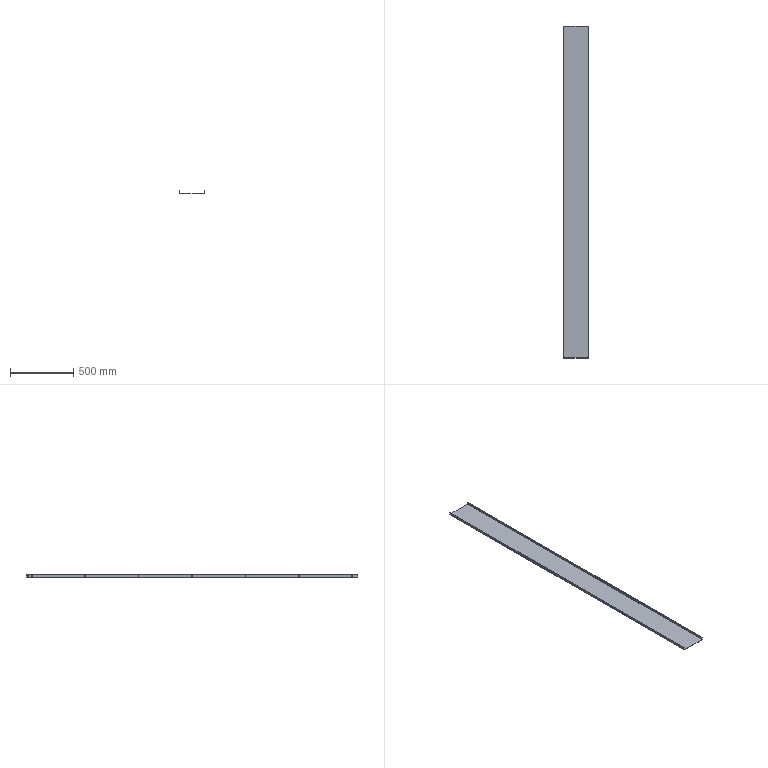Part | 1 solid | 64 faces | box 200 x 2616 x 20 mm | volume 926073 mm3 | cylinder 32 | plane 32 | commonest cylinder face diameters 6.2 x28 0.4 x2 3.4 x2